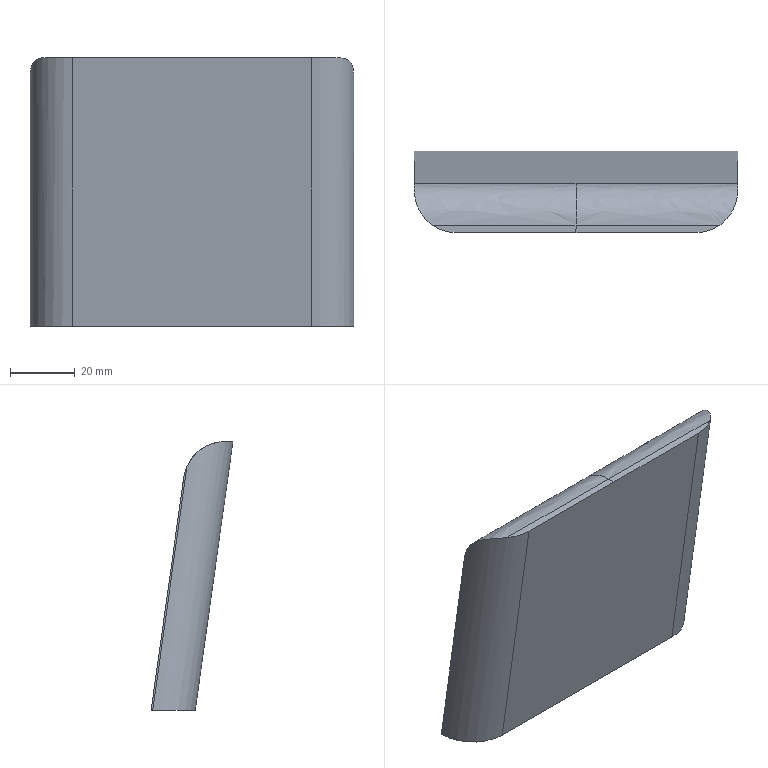Part | STEP file | solid 116 | 1 solid | 11 faces | box 100 x 25.292 x 82.969 mm | volume 104423 mm3 | plane 5 | spline 4 | cylinder 2 | commonest cylinder face diameters 26 x2